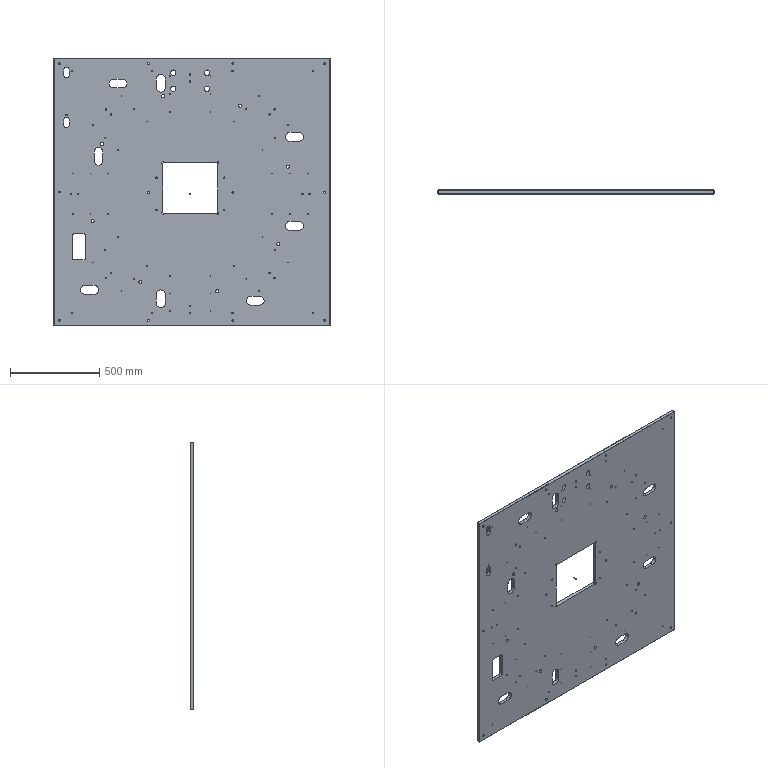Part | STEP file | 09-01 table plate | 2 solids | 550 faces | box 1550 x 20 x 1500 mm | volume 43532638 mm3 | cylinder 345 | cone 111 | plane 94 | commonest cylinder face diameters 5 x96 3.3 x72 18 x40 8 x32 11 x24 50 x19